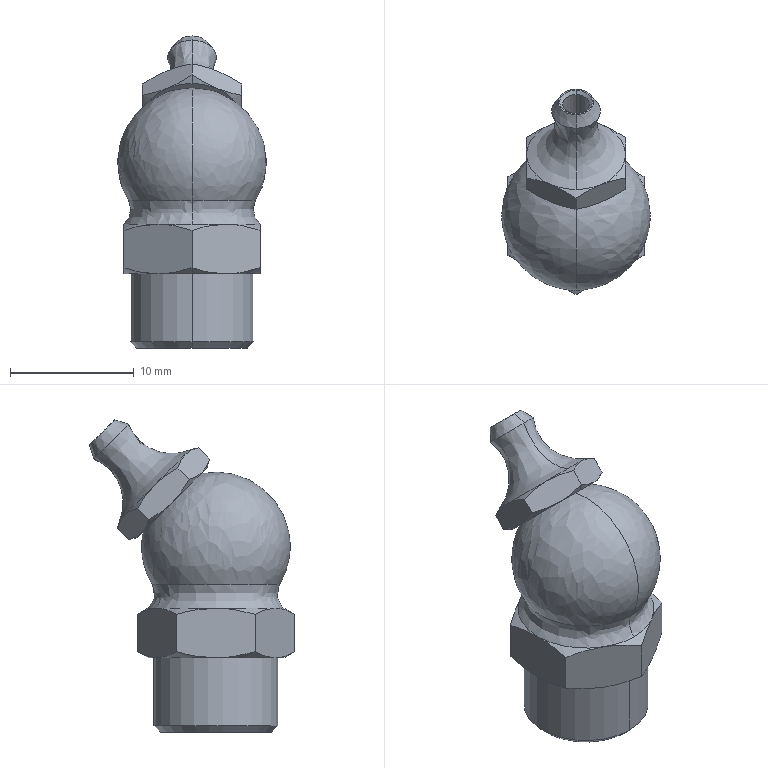Part | STEP file | Grease fitting_M10X1_45 | 1 solid | 74 faces | box 12 x 16.561 x 25.211 mm | volume 1753 mm3 | cone 38 | plane 21 | cylinder 9 | spline 6 | commonest cylinder face diameters 5 x4 2.16 x2 10 x2 2.88 x1